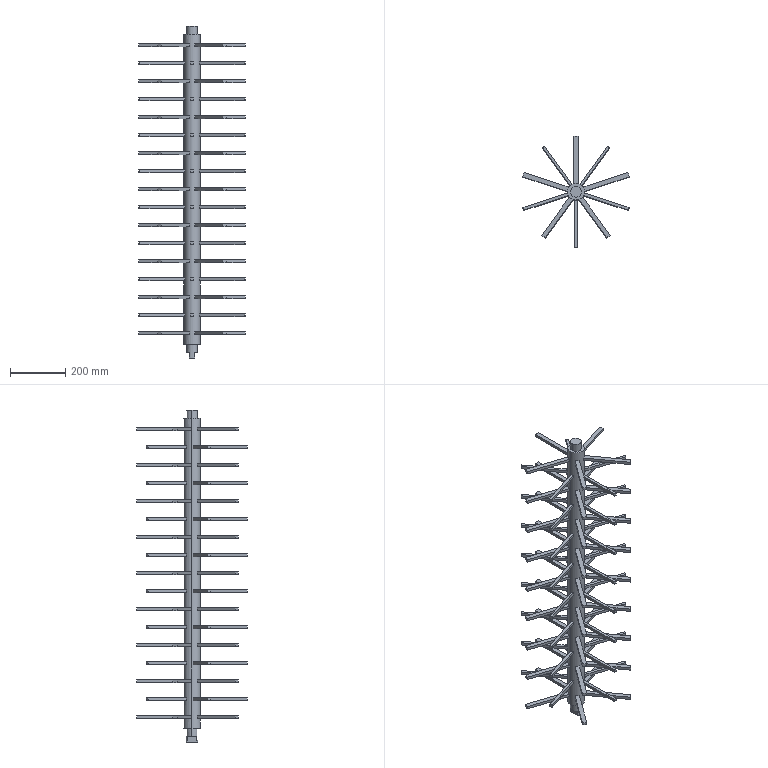Part | SolidWorks | 1 solid | 439 faces | box 385.062 x 400 x 1200 mm | volume 5164108 mm3 | plane 348 | cylinder 91 | commonest cylinder face diameters 400 x85 40 x4 60 x2